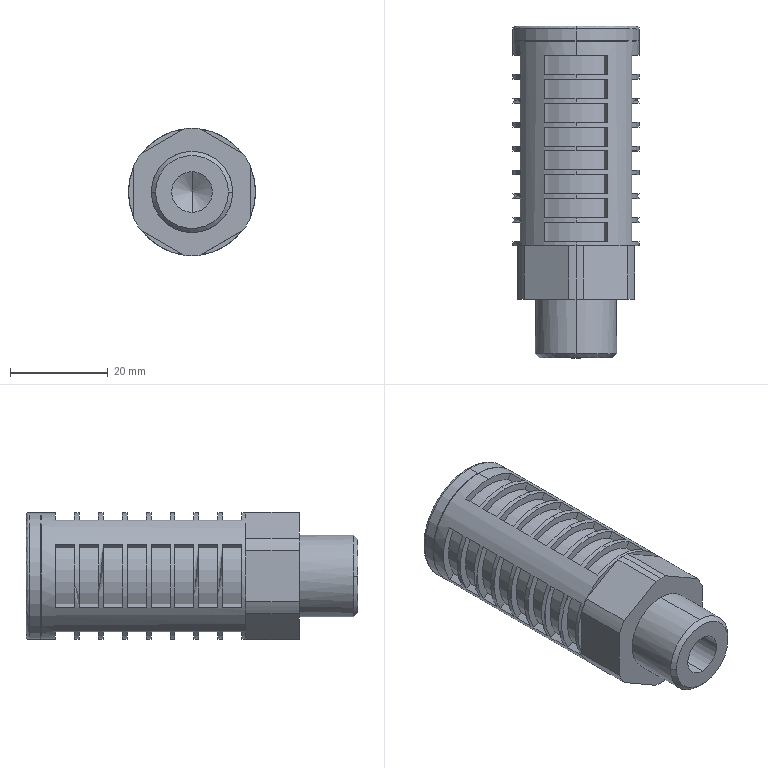Part | STEP file | plastic foam silencer PAL-03 | 1 solid | 205 faces | box 26 x 68 x 26.213 mm | volume 26024 mm3 | plane 150 | cylinder 47 | spline 4 | cone 4 | commonest cylinder face diameters 23 x32 26.213 x7 26 x4 8.331 x2 16.662 x2